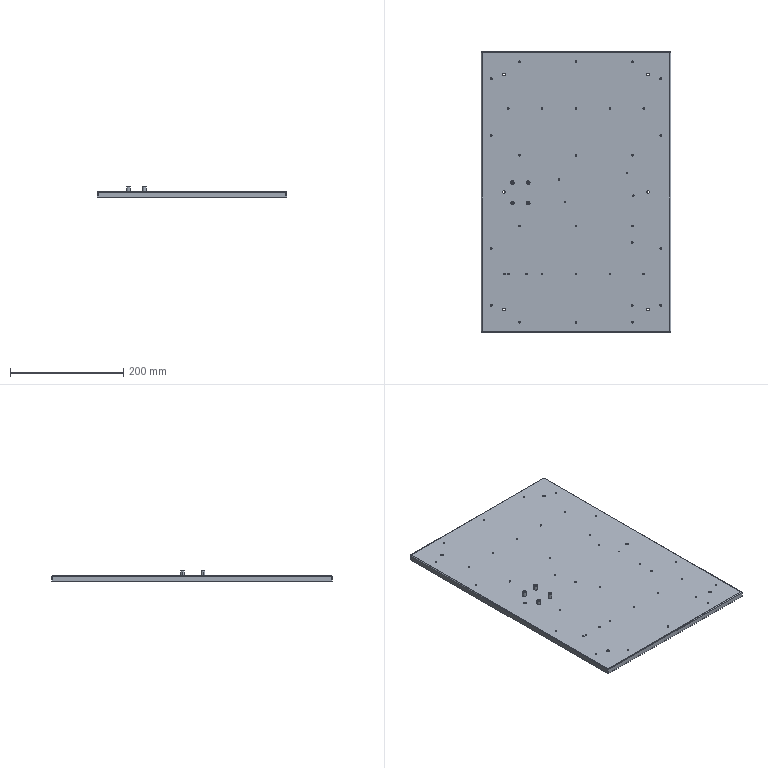Part | STEP file | 1 solid | 158 faces | box 335 x 495 x 18 mm | volume 269254 mm3 | cylinder 112 | plane 38 | cone 8 | commonest cylinder face diameters 3.3 x68 2.5 x16 4.8 x12 6.4 x8 0.02 x4 3.02 x4